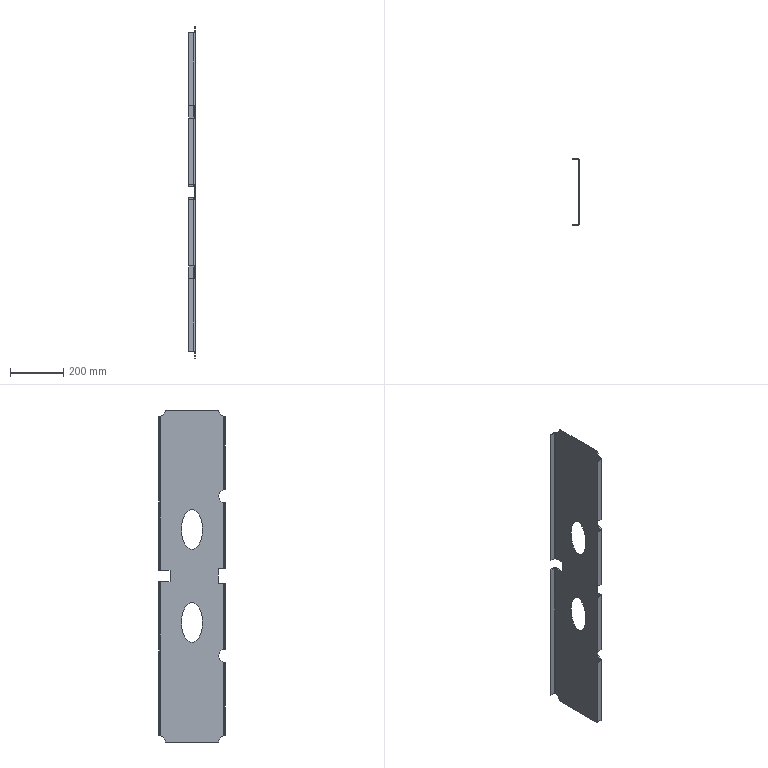Part | STEP file | VD-SYL0380DJ1006_1_2_1-3_STEP | 1 solid | 66 faces | box 25 x 251 x 1248 mm | volume 994019 mm3 | plane 36 | cylinder 18 | spline 12 | commonest cylinder face diameters 6 x6 12 x6 50 x6